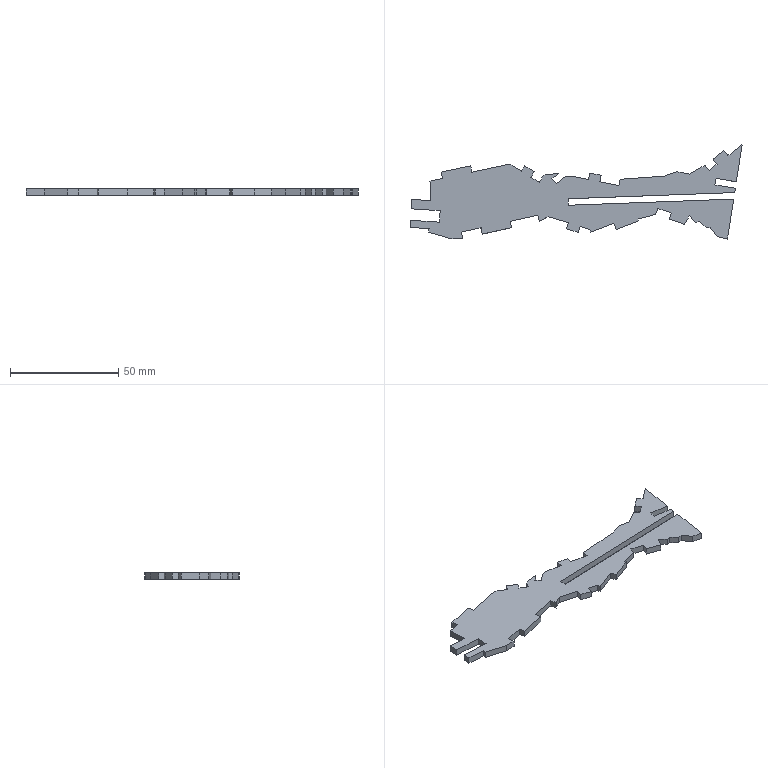Part | SolidWorks | features BaseBody 1 | 1 solid | 86 faces | box 153.331 x 43.468 x 3 mm | volume 9745 mm3 | plane 70 | spline 16